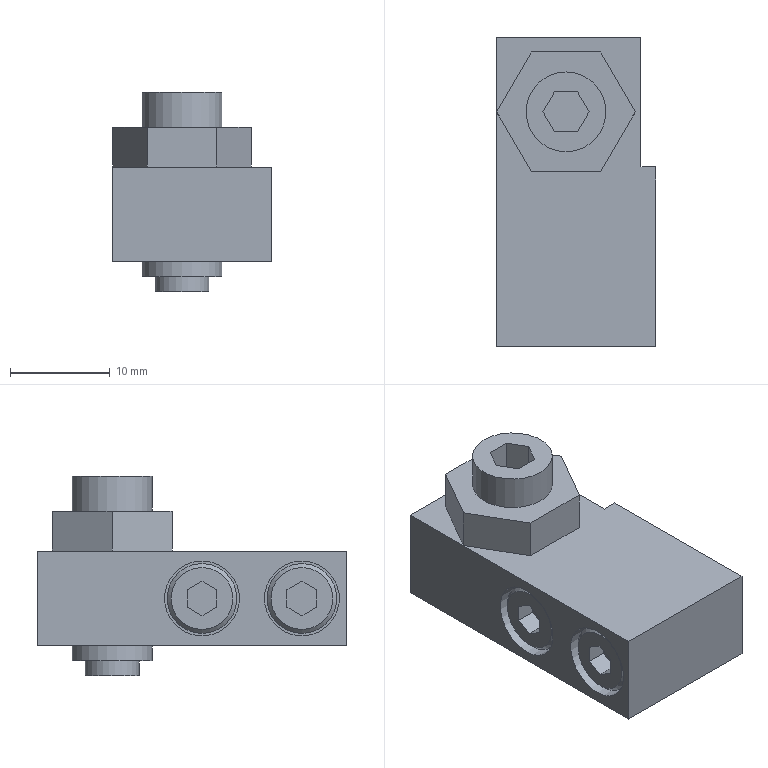Part | NX | 1 solid | 52 faces | box 16 x 31 x 20 mm | volume 5140 mm3 | plane 43 | cylinder 7 | cone 2 | commonest cylinder face diameters 7 x2 7.5 x2 8 x2 5.4 x1
STEP:
#1=CARTESIAN_POINT('',(-40.,0.5,58.5));
#2=VERTEX_POINT('',#1);
#3=CARTESIAN_POINT('',(-24.,0.5,58.5));
#4=VERTEX_POINT('',#3);
#5=CARTESIAN_POINT('',(-24.,0.5,58.5));
#6=DIRECTION('',(1.,0.,0.));
#7=VECTOR('',#6,1000.);
#8=LINE('',#5,#7);
#9=EDGE_CURVE('',#2,#4,#8,.T.);
#10=ORIENTED_EDGE('',*,*,#9,.F.);
#11=CARTESIAN_POINT('',(-40.,31.5,58.5));
#12=VERTEX_POINT('',#11);
#13=CARTESIAN_POINT('',(-40.,0.5,58.5));
#14=DIRECTION('',(0.,1.,0.));
#15=VECTOR('',#14,1000.);
#16=LINE('',#13,#15);
#17=EDGE_CURVE('',#12,#2,#16,.F.);
#18=ORIENTED_EDGE('',*,*,#17,.F.);
#19=CARTESIAN_POINT('',(-25.5,31.5,58.5));
#20=VERTEX_POINT('',#19);
#21=CARTESIAN_POINT('',(-24.,31.5,58.5));
#22=DIRECTION('',(1.,0.,0.));
#23=VECTOR('',#22,1000.);
#24=LINE('',#21,#23);
#25=EDGE_CURVE('',#20,#12,#24,.F.);
#26=ORIENTED_EDGE('',*,*,#25,.F.);
#27=CARTESIAN_POINT('',(-25.5,18.5,58.5));
#28=VERTEX_POINT('',#27);
#29=CARTESIAN_POINT('',(-25.5,0.5,58.5));
#30=DIRECTION('',(0.,1.,0.));
#31=VECTOR('',#30,1000.);
#32=LINE('',#29,#31);
#33=EDGE_CURVE('',#28,#20,#32,.T.);
#34=ORIENTED_EDGE('',*,*,#33,.F.);
#35=CARTESIAN_POINT('',(-24.,18.5,58.5));
#36=VERTEX_POINT('',#35);
#37=CARTESIAN_POINT('',(-24.,18.5,58.5));
#38=DIRECTION('',(1.,0.,0.));
#39=VECTOR('',#38,1000.);
#40=LINE('',#37,#39);
#41=EDGE_CURVE('',#36,#28,#40,.F.);
#42=ORIENTED_EDGE('',*,*,#41,.F.);
#43=CARTESIAN_POINT('',(-24.,0.5,58.5));
#44=DIRECTION('',(0.,1.,0.));
#45=VECTOR('',#44,1000.);
#46=LINE('',#43,#45);
#47=EDGE_CURVE('',#4,#36,#46,.T.);
#48=ORIENTED_EDGE('',*,*,#47,.F.);
#49=EDGE_LOOP('',(#10,#18,#26,#34,#42,#48));
#50=FACE_BOUND('',#49,.T.);
#51=CARTESIAN_POINT('',(-33.,28.,58.5));
#52=VERTEX_POINT('',#51);
#53=CARTESIAN_POINT('',(-33.,24.,58.5));
#54=DIRECTION('',(0.,0.,-1.));
#55=DIRECTION('',(0.,1.,0.));
#56=AXIS2_PLACEMENT_3D('',#53,#54,#55);
#57=CIRCLE('',#56,4.);
#58=EDGE_CURVE('',#52,#52,#57,.T.);
#59=ORIENTED_EDGE('',*,*,#58,.F.);
#60=EDGE_LOOP('',(#59));
#61=FACE_BOUND('',#60,.T.);
#62=CARTESIAN_POINT('',(-24.,0.5,58.5));
#63=DIRECTION('',(0.,0.,1.));
#64=DIRECTION('',(1.,0.,0.));
#65=AXIS2_PLACEMENT_3D('',#62,#63,#64);
#66=PLANE('',#65);
#67=ADVANCED_FACE('',(#50,#61),#66,.F.);
#68=CARTESIAN_POINT('',(-24.,18.5,68.));
#69=VERTEX_POINT('',#68);
#70=CARTESIAN_POINT('',(-24.,0.5,68.));
#71=VERTEX_POINT('',#70);
#72=CARTESIAN_POINT('',(-24.,0.5,68.));
#73=DIRECTION('',(0.,1.,0.));
#74=VECTOR('',#73,1000.);
#75=LINE('',#72,#74);
#76=EDGE_CURVE('',#69,#71,#75,.F.);
#77=ORIENTED_EDGE('',*,*,#76,.T.);
#78=CARTESIAN_POINT('',(-24.,0.5,68.));
#79=DIRECTION('',(0.,0.,-1.));
#80=VECTOR('',#79,1000.);
#81=LINE('',#78,#80);
#82=EDGE_CURVE('',#71,#4,#81,.T.);
#83=ORIENTED_EDGE('',*,*,#82,.T.);
#84=ORIENTED_EDGE('',*,*,#47,.T.);
#85=CARTESIAN_POINT('',(-24.,18.5,68.));
#86=DIRECTION('',(0.,0.,-1.));
#87=VECTOR('',#86,1000.);
#88=LINE('',#85,#87);
#89=EDGE_CURVE('',#36,#69,#88,.F.);
#90=ORIENTED_EDGE('',*,*,#89,.T.);
#91=EDGE_LOOP('',(#77,#83,#84,#90));
#92=FACE_BOUND('',#91,.T.);
#93=CARTESIAN_POINT('',(-24.,0.5,68.));
#94=DIRECTION('',(1.,0.,0.));
#95=DIRECTION('',(0.,0.,-1.));
#96=AXIS2_PLACEMENT_3D('',#93,#94,#95);
#97=PLANE('',#96);
#98=ADVANCED_FACE('',(#92),#97,.T.);
#99=CARTESIAN_POINT('',(-40.,0.5,68.));
#100=VERTEX_POINT('',#99);
#101=CARTESIAN_POINT('',(-40.,0.5,68.));
#102=DIRECTION('',(1.,0.,0.));
#103=VECTOR('',#102,1000.);
#104=LINE('',#101,#103);
#105=EDGE_CURVE('',#71,#100,#104,.F.);
#106=ORIENTED_EDGE('',*,*,#105,.T.);
#107=CARTESIAN_POINT('',(-40.,0.5,68.));
#108=DIRECTION('',(0.,0.,-1.));
#109=VECTOR('',#108,1000.);
#110=LINE('',#107,#109);
#111=EDGE_CURVE('',#100,#2,#110,.T.);
#112=ORIENTED_EDGE('',*,*,#111,.T.);
#113=ORIENTED_EDGE('',*,*,#9,.T.);
#114=ORIENTED_EDGE('',*,*,#82,.F.);
#115=EDGE_LOOP('',(#106,#112,#113,#114));
#116=FACE_BOUND('',#115,.T.);
#117=CARTESIAN_POINT('',(-40.,0.5,68.));
#118=DIRECTION('',(0.,-1.,0.));
#119=DIRECTION('',(0.,0.,-1.));
#120=AXIS2_PLACEMENT_3D('',#117,#118,#119);
#121=PLANE('',#120);
#122=ADVANCED_FACE('',(#116),#121,.T.);
#123=CARTESIAN_POINT('',(-40.,31.5,68.));
#124=VERTEX_POINT('',#123);
#125=CARTESIAN_POINT('',(-40.,31.5,68.));
#126=DIRECTION('',(0.,1.,0.));
#127=VECTOR('',#126,1000.);
#128=LINE('',#125,#127);
#129=EDGE_CURVE('',#100,#124,#128,.T.);
#130=ORIENTED_EDGE('',*,*,#129,.T.);
#131=CARTESIAN_POINT('',(-40.,31.5,68.));
#132=DIRECTION('',(0.,0.,1.));
#133=VECTOR('',#132,1000.);
#134=LINE('',#131,#133);
#135=EDGE_CURVE('',#124,#12,#134,.F.);
#136=ORIENTED_EDGE('',*,*,#135,.T.);
#137=ORIENTED_EDGE('',*,*,#17,.T.);
#138=ORIENTED_EDGE('',*,*,#111,.F.);
#139=EDGE_LOOP('',(#130,#136,#137,#138));
#140=FACE_BOUND('',#139,.T.);
#141=CARTESIAN_POINT('',(-40.,5.,67.));
#142=VERTEX_POINT('',#141);
#143=CARTESIAN_POINT('',(-40.,5.,63.25));
#144=DIRECTION('',(-1.,0.,0.));
#145=DIRECTION('',(0.,0.,1.));
#146=AXIS2_PLACEMENT_3D('',#143,#144,#145);
#147=CIRCLE('',#146,3.75);
#148=EDGE_CURVE('',#142,#142,#147,.F.);
#149=ORIENTED_EDGE('',*,*,#148,.T.);
#150=EDGE_LOOP('',(#149));
#151=FACE_BOUND('',#150,.T.);
#152=CARTESIAN_POINT('',(-40.,15.,67.));
#153=VERTEX_POINT('',#152);
#154=CARTESIAN_POINT('',(-40.,15.,63.25));
#155=DIRECTION('',(-1.,0.,0.));
#156=DIRECTION('',(0.,0.,1.));
#157=AXIS2_PLACEMENT_3D('',#154,#155,#156);
#158=CIRCLE('',#157,3.75);
#159=EDGE_CURVE('',#153,#153,#158,.F.);
#160=ORIENTED_EDGE('',*,*,#159,.T.);
#161=EDGE_LOOP('',(#160));
#162=FACE_BOUND('',#161,.T.);
#163=CARTESIAN_POINT('',(-40.,31.5,68.));
#164=DIRECTION('',(-1.,0.,0.));
#165=DIRECTION('',(0.,0.,1.));
#166=AXIS2_PLACEMENT_3D('',#163,#164,#165);
#167=PLANE('',#166);
#168=ADVANCED_FACE('',(#140,#151,#162),#167,.T.);
#169=CARTESIAN_POINT('',(-25.5,31.5,68.));
#170=VERTEX_POINT('',#169);
#171=CARTESIAN_POINT('',(-25.5,31.5,68.));
#172=DIRECTION('',(1.,0.,0.));
#173=VECTOR('',#172,1000.);
#174=LINE('',#171,#173);
#175=EDGE_CURVE('',#124,#170,#174,.T.);
#176=ORIENTED_EDGE('',*,*,#175,.T.);
#177=CARTESIAN_POINT('',(-25.5,31.5,68.));
#178=DIRECTION('',(0.,0.,1.));
#179=VECTOR('',#178,1000.);
#180=LINE('',#177,#179);
#181=EDGE_CURVE('',#170,#20,#180,.F.);
#182=ORIENTED_EDGE('',*,*,#181,.T.);
#183=ORIENTED_EDGE('',*,*,#25,.T.);
#184=ORIENTED_EDGE('',*,*,#135,.F.);
#185=EDGE_LOOP('',(#176,#182,#183,#184));
#186=FACE_BOUND('',#185,.T.);
#187=CARTESIAN_POINT('',(-25.5,31.5,68.));
#188=DIRECTION('',(0.,1.,0.));
#189=DIRECTION('',(0.,0.,1.));
#190=AXIS2_PLACEMENT_3D('',#187,#188,#189);
#191=PLANE('',#190);
#192=ADVANCED_FACE('',(#186),#191,.T.);
#193=CARTESIAN_POINT('',(-25.5,18.5,68.));
#194=VERTEX_POINT('',#193);
#195=CARTESIAN_POINT('',(-25.5,18.5,68.));
#196=DIRECTION('',(0.,1.,0.));
#197=VECTOR('',#196,1000.);
#198=LINE('',#195,#197);
#199=EDGE_CURVE('',#170,#194,#198,.F.);
#200=ORIENTED_EDGE('',*,*,#199,.T.);
#201=CARTESIAN_POINT('',(-25.5,18.5,68.));
#202=DIRECTION('',(0.,0.,-1.));
#203=VECTOR('',#202,1000.);
#204=LINE('',#201,#203);
#205=EDGE_CURVE('',#194,#28,#204,.T.);
#206=ORIENTED_EDGE('',*,*,#205,.T.);
#207=ORIENTED_EDGE('',*,*,#33,.T.);
#208=ORIENTED_EDGE('',*,*,#181,.F.);
#209=EDGE_LOOP('',(#200,#206,#207,#208));
#210=FACE_BOUND('',#209,.T.);
#211=CARTESIAN_POINT('',(-25.5,18.5,68.));
#212=DIRECTION('',(1.,0.,0.));
#213=DIRECTION('',(0.,0.,-1.));
#214=AXIS2_PLACEMENT_3D('',#211,#212,#213);
#215=PLANE('',#214);
#216=ADVANCED_FACE('',(#210),#215,.T.);
#217=CARTESIAN_POINT('',(-33.,28.,57.));
#218=VERTEX_POINT('',#217);
#219=CARTESIAN_POINT('',(-33.,24.,57.));
#220=DIRECTION('',(0.,0.,-1.));
#221=DIRECTION('',(0.,1.,0.));
#222=AXIS2_PLACEMENT_3D('',#219,#220,#221);
#223=CIRCLE('',#222,4.);
#224=EDGE_CURVE('',#218,#218,#223,.F.);
#225=ORIENTED_EDGE('',*,*,#224,.T.);
#226=EDGE_LOOP('',(#225));
#227=FACE_BOUND('',#226,.T.);
#228=ORIENTED_EDGE('',*,*,#58,.T.);
#229=EDGE_LOOP('',(#228));
#230=FACE_BOUND('',#229,.T.);
#231=CARTESIAN_POINT('',(-33.,24.,66.25));
#232=DIRECTION('',(0.,0.,-1.));
#233=DIRECTION('',(0.,1.,0.));
#234=AXIS2_PLACEMENT_3D('',#231,#232,#233);
#235=CYLINDRICAL_SURFACE('',#234,4.);
#236=ADVANCED_FACE('',(#227,#230),#235,.T.);
#237=ORIENTED_EDGE('',*,*,#175,.F.);
#238=ORIENTED_EDGE('',*,*,#129,.F.);
#239=ORIENTED_EDGE('',*,*,#105,.F.);
#240=ORIENTED_EDGE('',*,*,#76,.F.);
#241=CARTESIAN_POINT('',(-24.,18.5,68.));
#242=DIRECTION('',(1.,0.,0.));
#243=VECTOR('',#242,1000.);
#244=LINE('',#241,#243);
#245=EDGE_CURVE('',#69,#194,#244,.F.);
#246=ORIENTED_EDGE('',*,*,#245,.T.);
#247=ORIENTED_EDGE('',*,*,#199,.F.);
#248=EDGE_LOOP('',(#237,#238,#239,#240,#246,#247));
#249=FACE_BOUND('',#248,.T.);
#250=CARTESIAN_POINT('',(-29.536,18.,68.));
#251=VERTEX_POINT('',#250);
#252=CARTESIAN_POINT('',(-36.464,18.,68.));
#253=VERTEX_POINT('',#252);
#254=CARTESIAN_POINT('',(-24.,18.,68.));
#255=DIRECTION('',(1.,0.,0.));
#256=VECTOR('',#255,1000.);
#257=LINE('',#254,#256);
#258=EDGE_CURVE('',#251,#253,#257,.F.);
#259=ORIENTED_EDGE('',*,*,#258,.T.);
#260=CARTESIAN_POINT('',(-39.928,24.,68.));
#261=VERTEX_POINT('',#260);
#262=CARTESIAN_POINT('',(-36.464,18.,68.));
#263=DIRECTION('',(-0.5,0.866,0.));
#264=VECTOR('',#263,1000.);
#265=LINE('',#262,#264);
#266=EDGE_CURVE('',#253,#261,#265,.T.);
#267=ORIENTED_EDGE('',*,*,#266,.T.);
#268=CARTESIAN_POINT('',(-36.464,30.,68.));
#269=VERTEX_POINT('',#268);
#270=CARTESIAN_POINT('',(-39.928,24.,68.));
#271=DIRECTION('',(0.5,0.866,0.));
#272=VECTOR('',#271,1000.);
#273=LINE('',#270,#272);
#274=EDGE_CURVE('',#261,#269,#273,.T.);
#275=ORIENTED_EDGE('',*,*,#274,.T.);
#276=CARTESIAN_POINT('',(-29.536,30.,68.));
#277=VERTEX_POINT('',#276);
#278=CARTESIAN_POINT('',(-24.,30.,68.));
#279=DIRECTION('',(1.,0.,0.));
#280=VECTOR('',#279,1000.);
#281=LINE('',#278,#280);
#282=EDGE_CURVE('',#269,#277,#281,.T.);
#283=ORIENTED_EDGE('',*,*,#282,.T.);
#284=CARTESIAN_POINT('',(-26.072,24.,68.));
#285=VERTEX_POINT('',#284);
#286=CARTESIAN_POINT('',(-29.536,30.,68.));
#287=DIRECTION('',(0.5,-0.866,0.));
#288=VECTOR('',#287,1000.);
#289=LINE('',#286,#288);
#290=EDGE_CURVE('',#277,#285,#289,.T.);
#291=ORIENTED_EDGE('',*,*,#290,.T.);
#292=CARTESIAN_POINT('',(-26.072,24.,68.));
#293=DIRECTION('',(-0.5,-0.866,0.));
#294=VECTOR('',#293,1000.);
#295=LINE('',#292,#294);
#296=EDGE_CURVE('',#285,#251,#295,.T.);
#297=ORIENTED_EDGE('',*,*,#296,.T.);
#298=EDGE_LOOP('',(#259,#267,#275,#283,#291,#297));
#299=FACE_BOUND('',#298,.T.);
#300=CARTESIAN_POINT('',(-24.,0.5,68.));
#301=DIRECTION('',(0.,0.,1.));
#302=DIRECTION('',(1.,0.,0.));
#303=AXIS2_PLACEMENT_3D('',#300,#301,#302);
#304=PLANE('',#303);
#305=ADVANCED_FACE('',(#249,#299),#304,.T.);
#306=ORIENTED_EDGE('',*,*,#245,.F.);
#307=ORIENTED_EDGE('',*,*,#89,.F.);
#308=ORIENTED_EDGE('',*,*,#41,.T.);
#309=ORIENTED_EDGE('',*,*,#205,.F.);
#310=EDGE_LOOP('',(#306,#307,#308,#309));
#311=FACE_BOUND('',#310,.T.);
#312=CARTESIAN_POINT('',(-24.,18.5,68.));
#313=DIRECTION('',(0.,1.,0.));
#314=DIRECTION('',(0.,0.,1.));
#315=AXIS2_PLACEMENT_3D('',#312,#313,#314);
#316=PLANE('',#315);
#317=ADVANCED_FACE('',(#311),#316,.T.);
#318=ORIENTED_EDGE('',*,*,#148,.F.);
#319=EDGE_LOOP('',(#318));
#320=FACE_BOUND('',#319,.T.);
#321=CARTESIAN_POINT('',(-35.6,5.,67.));
#322=VERTEX_POINT('',#321);
#323=CARTESIAN_POINT('',(-35.6,5.,63.25));
#324=DIRECTION('',(-1.,0.,0.));
#325=DIRECTION('',(0.,0.,1.));
#326=AXIS2_PLACEMENT_3D('',#323,#324,#325);
#327=CIRCLE('',#326,3.75);
#328=EDGE_CURVE('',#322,#322,#327,.T.);
#329=ORIENTED_EDGE('',*,*,#328,.F.);
#330=EDGE_LOOP('',(#329));
#331=FACE_BOUND('',#330,.T.);
#332=CARTESIAN_POINT('',(-40.,5.,63.25));
#333=DIRECTION('',(-1.,0.,0.));
#334=DIRECTION('',(0.,0.,1.));
#335=AXIS2_PLACEMENT_3D('',#332,#333,#334);
#336=CYLINDRICAL_SURFACE('',#335,3.75);
#337=ADVANCED_FACE('',(#320,#331),#336,.F.);
#338=ORIENTED_EDGE('',*,*,#159,.F.);
#339=EDGE_LOOP('',(#338));
#340=FACE_BOUND('',#339,.T.);
#341=CARTESIAN_POINT('',(-35.6,15.,67.));
#342=VERTEX_POINT('',#341);
#343=CARTESIAN_POINT('',(-35.6,15.,63.25));
#344=DIRECTION('',(-1.,0.,0.));
#345=DIRECTION('',(0.,0.,1.));
#346=AXIS2_PLACEMENT_3D('',#343,#344,#345);
#347=CIRCLE('',#346,3.75);
#348=EDGE_CURVE('',#342,#342,#347,.T.);
#349=ORIENTED_EDGE('',*,*,#348,.F.);
#350=EDGE_LOOP('',(#349));
#351=FACE_BOUND('',#350,.T.);
#352=CARTESIAN_POINT('',(-40.,15.,63.25));
#353=DIRECTION('',(-1.,0.,0.));
#354=DIRECTION('',(0.,0.,1.));
#355=AXIS2_PLACEMENT_3D('',#352,#353,#354);
#356=CYLINDRICAL_SURFACE('',#355,3.75);
#357=ADVANCED_FACE('',(#340,#351),#356,.F.);
#358=CARTESIAN_POINT('',(-33.,26.7,57.));
#359=VERTEX_POINT('',#358);
#360=CARTESIAN_POINT('',(-33.,24.,57.));
#361=DIRECTION('',(0.,0.,-1.));
#362=DIRECTION('',(0.,1.,0.));
#363=AXIS2_PLACEMENT_3D('',#360,#361,#362);
#364=CIRCLE('',#363,2.7);
#365=EDGE_CURVE('',#359,#359,#364,.F.);
#366=ORIENTED_EDGE('',*,*,#365,.T.);
#367=EDGE_LOOP('',(#366));
#368=FACE_BOUND('',#367,.T.);
#369=ORIENTED_EDGE('',*,*,#224,.F.);
#370=EDGE_LOOP('',(#369));
#371=FACE_BOUND('',#370,.T.);
#372=CARTESIAN_POINT('',(-33.,27.35,57.));
#373=DIRECTION('',(0.,0.,-1.));
#374=DIRECTION('',(-1.,0.,0.));
#375=AXIS2_PLACEMENT_3D('',#372,#373,#374);
#376=PLANE('',#375);
#377=ADVANCED_FACE('',(#368,#371),#376,.T.);
#378=ORIENTED_EDGE('',*,*,#266,.F.);
#379=CARTESIAN_POINT('',(-36.464,18.,72.));
#380=VERTEX_POINT('',#379);
#381=CARTESIAN_POINT('',(-36.464,18.,68.));
#382=DIRECTION('',(0.,0.,1.));
#383=VECTOR('',#382,1000.);
#384=LINE('',#381,#383);
#385=EDGE_CURVE('',#253,#380,#384,.T.);
#386=ORIENTED_EDGE('',*,*,#385,.T.);
#387=CARTESIAN_POINT('',(-39.928,24.,72.));
#388=VERTEX_POINT('',#387);
#389=CARTESIAN_POINT('',(-36.464,18.,72.));
#390=DIRECTION('',(0.5,-0.866,0.));
#391=VECTOR('',#390,1000.);
#392=LINE('',#389,#391);
#393=EDGE_CURVE('',#380,#388,#392,.F.);
#394=ORIENTED_EDGE('',*,*,#393,.T.);
#395=CARTESIAN_POINT('',(-39.928,24.,68.));
#396=DIRECTION('',(0.,0.,1.));
#397=VECTOR('',#396,1000.);
#398=LINE('',#395,#397);
#399=EDGE_CURVE('',#388,#261,#398,.F.);
#400=ORIENTED_EDGE('',*,*,#399,.T.);
#401=EDGE_LOOP('',(#378,#386,#394,#400));
#402=FACE_BOUND('',#401,.T.);
#403=CARTESIAN_POINT('',(-36.464,18.,68.));
#404=DIRECTION('',(-0.866,-0.5,0.));
#405=DIRECTION('',(0.5,-0.866,0.));
#406=AXIS2_PLACEMENT_3D('',#403,#404,#405);
#407=PLANE('',#406);
#408=ADVANCED_FACE('',(#402),#407,.T.);
#409=ORIENTED_EDGE('',*,*,#258,.F.);
#410=CARTESIAN_POINT('',(-29.536,18.,72.));
#411=VERTEX_POINT('',#410);
#412=CARTESIAN_POINT('',(-29.536,18.,68.));
#413=DIRECTION('',(0.,0.,1.));
#414=VECTOR('',#413,1000.);
#415=LINE('',#412,#414);
#416=EDGE_CURVE('',#251,#411,#415,.T.);
#417=ORIENTED_EDGE('',*,*,#416,.T.);
#418=CARTESIAN_POINT('',(-29.536,18.,72.));
#419=DIRECTION('',(1.,0.,0.));
#420=VECTOR('',#419,1000.);
#421=LINE('',#418,#420);
#422=EDGE_CURVE('',#411,#380,#421,.F.);
#423=ORIENTED_EDGE('',*,*,#422,.T.);
#424=ORIENTED_EDGE('',*,*,#385,.F.);
#425=EDGE_LOOP('',(#409,#417,#423,#424));
#426=FACE_BOUND('',#425,.T.);
#427=CARTESIAN_POINT('',(-29.536,18.,68.));
#428=DIRECTION('',(0.,-1.,0.));
#429=DIRECTION('',(1.,0.,0.));
#430=AXIS2_PLACEMENT_3D('',#427,#428,#429);
#431=PLANE('',#430);
#432=ADVANCED_FACE('',(#426),#431,.T.);
#433=ORIENTED_EDGE('',*,*,#296,.F.);
#434=CARTESIAN_POINT('',(-26.072,24.,72.));
#435=VERTEX_POINT('',#434);
#436=CARTESIAN_POINT('',(-26.072,24.,68.));
#437=DIRECTION('',(0.,0.,1.));
#438=VECTOR('',#437,1000.);
#439=LINE('',#436,#438);
#440=EDGE_CURVE('',#285,#435,#439,.T.);
#441=ORIENTED_EDGE('',*,*,#440,.T.);
#442=CARTESIAN_POINT('',(-26.072,24.,72.));
#443=DIRECTION('',(0.5,0.866,0.));
#444=VECTOR('',#443,1000.);
#445=LINE('',#442,#444);
#446=EDGE_CURVE('',#435,#411,#445,.F.);
#447=ORIENTED_EDGE('',*,*,#446,.T.);
#448=ORIENTED_EDGE('',*,*,#416,.F.);
#449=EDGE_LOOP('',(#433,#441,#447,#448));
#450=FACE_BOUND('',#449,.T.);
#451=CARTESIAN_POINT('',(-26.072,24.,68.));
#452=DIRECTION('',(0.866,-0.5,0.));
#453=DIRECTION('',(0.5,0.866,0.));
#454=AXIS2_PLACEMENT_3D('',#451,#452,#453);
#455=PLANE('',#454);
#456=ADVANCED_FACE('',(#450),#455,.T.);
#457=ORIENTED_EDGE('',*,*,#290,.F.);
#458=CARTESIAN_POINT('',(-29.536,30.,72.));
#459=VERTEX_POINT('',#458);
#460=CARTESIAN_POINT('',(-29.536,30.,68.));
#461=DIRECTION('',(0.,0.,1.));
#462=VECTOR('',#461,1000.);
#463=LINE('',#460,#462);
#464=EDGE_CURVE('',#277,#459,#463,.T.);
#465=ORIENTED_EDGE('',*,*,#464,.T.);
#466=CARTESIAN_POINT('',(-29.536,30.,72.));
#467=DIRECTION('',(-0.5,0.866,0.));
#468=VECTOR('',#467,1000.);
#469=LINE('',#466,#468);
#470=EDGE_CURVE('',#459,#435,#469,.F.);
#471=ORIENTED_EDGE('',*,*,#470,.T.);
#472=ORIENTED_EDGE('',*,*,#440,.F.);
#473=EDGE_LOOP('',(#457,#465,#471,#472));
#474=FACE_BOUND('',#473,.T.);
#475=CARTESIAN_POINT('',(-29.536,30.,68.));
#476=DIRECTION('',(0.866,0.5,0.));
#477=DIRECTION('',(-0.5,0.866,0.));
#478=AXIS2_PLACEMENT_3D('',#475,#476,#477);
#479=PLANE('',#478);
#480=ADVANCED_FACE('',(#474),#479,.T.);
#481=ORIENTED_EDGE('',*,*,#282,.F.);
#482=CARTESIAN_POINT('',(-36.464,30.,72.));
#483=VERTEX_POINT('',#482);
#484=CARTESIAN_POINT('',(-36.464,30.,68.));
#485=DIRECTION('',(0.,0.,1.));
#486=VECTOR('',#485,1000.);
#487=LINE('',#484,#486);
#488=EDGE_CURVE('',#269,#483,#487,.T.);
#489=ORIENTED_EDGE('',*,*,#488,.T.);
#490=CARTESIAN_POINT('',(-36.464,30.,72.));
#491=DIRECTION('',(-1.,0.,0.));
#492=VECTOR('',#491,1000.);
#493=LINE('',#490,#492);
#494=EDGE_CURVE('',#483,#459,#493,.F.);
#495=ORIENTED_EDGE('',*,*,#494,.T.);
#496=ORIENTED_EDGE('',*,*,#464,.F.);
#497=EDGE_LOOP('',(#481,#489,#495,#496));
#498=FACE_BOUND('',#497,.T.);
#499=CARTESIAN_POINT('',(-36.464,30.,68.));
#500=DIRECTION('',(0.,1.,0.));
#501=DIRECTION('',(-1.,0.,0.));
#502=AXIS2_PLACEMENT_3D('',#499,#500,#501);
#503=PLANE('',#502);
#504=ADVANCED_FACE('',(#498),#503,.T.);
#505=ORIENTED_EDGE('',*,*,#274,.F.);
#506=ORIENTED_EDGE('',*,*,#399,.F.);
#507=CARTESIAN_POINT('',(-39.928,24.,72.));
#508=DIRECTION('',(-0.5,-0.866,0.));
#509=VECTOR('',#508,1000.);
#510=LINE('',#507,#509);
#511=EDGE_CURVE('',#388,#483,#510,.F.);
#512=ORIENTED_EDGE('',*,*,#511,.T.);
#513=ORIENTED_EDGE('',*,*,#488,.F.);
#514=EDGE_LOOP('',(#505,#506,#512,#513));
#515=FACE_BOUND('',#514,.T.);
#516=CARTESIAN_POINT('',(-39.928,24.,68.));
#517=DIRECTION('',(-0.866,0.5,0.));
#518=DIRECTION('',(-0.5,-0.866,0.));
#519=AXIS2_PLACEMENT_3D('',#516,#517,#518);
#520=PLANE('',#519);
#521=ADVANCED_FACE('',(#515),#520,.T.);
#522=ORIENTED_EDGE('',*,*,#328,.T.);
#523=EDGE_LOOP('',(#522));
#524=FACE_BOUND('',#523,.T.);
#525=CARTESIAN_POINT('',(-35.6,5.,66.75));
#526=VERTEX_POINT('',#525);
#527=CARTESIAN_POINT('',(-35.6,5.,63.25));
#528=DIRECTION('',(-1.,0.,0.));
#529=DIRECTION('',(0.,0.,1.));
#530=AXIS2_PLACEMENT_3D('',#527,#528,#529);
#531=CIRCLE('',#530,3.5);
#532=EDGE_CURVE('',#526,#526,#531,.T.);
#533=ORIENTED_EDGE('',*,*,#532,.F.);
#534=EDGE_LOOP('',(#533));
#535=FACE_BOUND('',#534,.T.);
#536=CARTESIAN_POINT('',(-35.6,0.5,63.25));
#537=DIRECTION('',(1.,0.,0.));
#538=DIRECTION('',(0.,0.,-1.));
#539=AXIS2_PLACEMENT_3D('',#536,#537,#538);
#540=PLANE('',#539);
#541=ADVANCED_FACE('',(#524,#535),#540,.F.);
#542=ORIENTED_EDGE('',*,*,#348,.T.);
#543=EDGE_LOOP('',(#542));
#544=FACE_BOUND('',#543,.T.);
#545=CARTESIAN_POINT('',(-35.6,15.,66.75));
#546=VERTEX_POINT('',#545);
#547=CARTESIAN_POINT('',(-35.6,15.,63.25));
#548=DIRECTION('',(-1.,0.,0.));
#549=DIRECTION('',(0.,0.,1.));
#550=AXIS2_PLACEMENT_3D('',#547,#548,#549);
#551=CIRCLE('',#550,3.5);
#552=EDGE_CURVE('',#546,#546,#551,.T.);
#553=ORIENTED_EDGE('',*,*,#552,.F.);
#554=EDGE_LOOP('',(#553));
#555=FACE_BOUND('',#554,.T.);
#556=CARTESIAN_POINT('',(-35.6,10.5,63.25));
#557=DIRECTION('',(1.,0.,0.));
#558=DIRECTION('',(0.,0.,-1.));
#559=AXIS2_PLACEMENT_3D('',#556,#557,#558);
#560=PLANE('',#559);
#561=ADVANCED_FACE('',(#544,#555),#560,.F.);
#562=ORIENTED_EDGE('',*,*,#365,.F.);
#563=EDGE_LOOP('',(#562));
#564=FACE_BOUND('',#563,.T.);
#565=CARTESIAN_POINT('',(-33.,26.7,55.5));
#566=VERTEX_POINT('',#565);
#567=CARTESIAN_POINT('',(-33.,24.,55.5));
#568=DIRECTION('',(0.,0.,-1.));
#569=DIRECTION('',(0.,1.,0.));
#570=AXIS2_PLACEMENT_3D('',#567,#568,#569);
#571=CIRCLE('',#570,2.7);
#572=EDGE_CURVE('',#566,#566,#571,.F.);
#573=ORIENTED_EDGE('',*,*,#572,.T.);
#574=EDGE_LOOP('',(#573));
#575=FACE_BOUND('',#574,.T.);
#576=CARTESIAN_POINT('',(-33.,24.,56.25));
#577=DIRECTION('',(0.,0.,-1.));
#578=DIRECTION('',(0.,1.,0.));
#579=AXIS2_PLACEMENT_3D('',#576,#577,#578);
#580=CYLINDRICAL_SURFACE('',#579,2.7);
#581=ADVANCED_FACE('',(#564,#575),#580,.T.);
#582=CARTESIAN_POINT('',(-33.,28.,72.));
#583=VERTEX_POINT('',#582);
#584=CARTESIAN_POINT('',(-33.,24.,72.));
#585=DIRECTION('',(0.,0.,-1.));
#586=DIRECTION('',(0.,1.,0.));
#587=AXIS2_PLACEMENT_3D('',#584,#585,#586);
#588=CIRCLE('',#587,4.);
#589=EDGE_CURVE('',#583,#583,#588,.T.);
#590=ORIENTED_EDGE('',*,*,#589,.T.);
#591=EDGE_LOOP('',(#590));
#592=FACE_BOUND('',#591,.T.);
#593=ORIENTED_EDGE('',*,*,#470,.F.);
#594=ORIENTED_EDGE('',*,*,#494,.F.);
#595=ORIENTED_EDGE('',*,*,#511,.F.);
#596=ORIENTED_EDGE('',*,*,#393,.F.);
#597=ORIENTED_EDGE('',*,*,#422,.F.);
#598=ORIENTED_EDGE('',*,*,#446,.F.);
#599=EDGE_LOOP('',(#593,#594,#595,#596,#597,#598));
#600=FACE_BOUND('',#599,.T.);
#601=CARTESIAN_POINT('',(-24.,0.5,72.));
#602=DIRECTION('',(0.,0.,1.));
#603=DIRECTION('',(1.,0.,0.));
#604=AXIS2_PLACEMENT_3D('',#601,#602,#603);
#605=PLANE('',#604);
#606=ADVANCED_FACE('',(#592,#600),#605,.T.);
#607=CARTESIAN_POINT('',(-39.2,5.,66.75));
#608=VERTEX_POINT('',#607);
#609=CARTESIAN_POINT('',(-39.2,5.,63.25));
#610=DIRECTION('',(-1.,0.,0.));
#611=DIRECTION('',(0.,0.,1.));
#612=AXIS2_PLACEMENT_3D('',#609,#610,#611);
#613=CIRCLE('',#612,3.5);
#614=EDGE_CURVE('',#608,#608,#613,.F.);
#615=ORIENTED_EDGE('',*,*,#614,.T.);
#616=EDGE_LOOP('',(#615));
#617=FACE_BOUND('',#616,.T.);
#618=ORIENTED_EDGE('',*,*,#532,.T.);
#619=EDGE_LOOP('',(#618));
#620=FACE_BOUND('',#619,.T.);
#621=CARTESIAN_POINT('',(-37.4,5.,63.25));
#622=DIRECTION('',(-1.,0.,0.));
#623=DIRECTION('',(0.,0.,1.));
#624=AXIS2_PLACEMENT_3D('',#621,#622,#623);
#625=CYLINDRICAL_SURFACE('',#624,3.5);
#626=ADVANCED_FACE('',(#617,#620),#625,.T.);
#627=CARTESIAN_POINT('',(-39.2,15.,66.75));
#628=VERTEX_POINT('',#627);
#629=CARTESIAN_POINT('',(-39.2,15.,63.25));
#630=DIRECTION('',(-1.,0.,0.));
#631=DIRECTION('',(0.,0.,1.));
#632=AXIS2_PLACEMENT_3D('',#629,#630,#631);
#633=CIRCLE('',#632,3.5);
#634=EDGE_CURVE('',#628,#628,#633,.F.);
#635=ORIENTED_EDGE('',*,*,#634,.T.);
#636=EDGE_LOOP('',(#635));
#637=FACE_BOUND('',#636,.T.);
#638=ORIENTED_EDGE('',*,*,#552,.T.);
#639=EDGE_LOOP('',(#638));
#640=FACE_BOUND('',#639,.T.);
#641=CARTESIAN_POINT('',(-37.4,15.,63.25));
#642=DIRECTION('',(-1.,0.,0.));
#643=DIRECTION('',(0.,0.,1.));
#644=AXIS2_PLACEMENT_3D('',#641,#642,#643);
#645=CYLINDRICAL_SURFACE('',#644,3.5);
#646=ADVANCED_FACE('',(#637,#640),#645,.T.);
#647=ORIENTED_EDGE('',*,*,#572,.F.);
#648=EDGE_LOOP('',(#647));
#649=FACE_BOUND('',#648,.T.);
#650=CARTESIAN_POINT('',(-33.,25.35,55.5));
#651=DIRECTION('',(0.,0.,-1.));
#652=DIRECTION('',(-1.,0.,0.));
#653=AXIS2_PLACEMENT_3D('',#650,#651,#652);
#654=PLANE('',#653);
#655=ADVANCED_FACE('',(#649),#654,.T.);
#656=ORIENTED_EDGE('',*,*,#589,.F.);
#657=EDGE_LOOP('',(#656));
#658=FACE_BOUND('',#657,.T.);
#659=CARTESIAN_POINT('',(-33.,28.,75.5));
#660=VERTEX_POINT('',#659);
#661=CARTESIAN_POINT('',(-33.,24.,75.5));
#662=DIRECTION('',(0.,0.,-1.));
#663=DIRECTION('',(0.,1.,0.));
#664=AXIS2_PLACEMENT_3D('',#661,#662,#663);
#665=CIRCLE('',#664,4.);
#666=EDGE_CURVE('',#660,#660,#665,.T.);
#667=ORIENTED_EDGE('',*,*,#666,.T.);
#668=EDGE_LOOP('',(#667));
#669=FACE_BOUND('',#668,.T.);
#670=CARTESIAN_POINT('',(-33.,24.,66.25));
#671=DIRECTION('',(0.,0.,-1.));
#672=DIRECTION('',(0.,1.,0.));
#673=AXIS2_PLACEMENT_3D('',#670,#671,#672);
#674=CYLINDRICAL_SURFACE('',#673,4.);
#675=ADVANCED_FACE('',(#658,#669),#674,.T.);
#676=CARTESIAN_POINT('',(-39.6,5.,60.15));
#677=VERTEX_POINT('',#676);
#678=CARTESIAN_POINT('',(-39.6,5.,63.25));
#679=DIRECTION('',(1.,0.,0.));
#680=DIRECTION('',(0.,0.,-1.));
#681=AXIS2_PLACEMENT_3D('',#678,#679,#680);
#682=CIRCLE('',#681,3.1);
#683=EDGE_CURVE('',#677,#677,#682,.T.);
#684=ORIENTED_EDGE('',*,*,#683,.T.);
#685=EDGE_LOOP('',(#684));
#686=FACE_BOUND('',#685,.T.);
#687=ORIENTED_EDGE('',*,*,#614,.F.);
#688=EDGE_LOOP('',(#687));
#689=FACE_BOUND('',#688,.T.);
#690=CARTESIAN_POINT('',(-39.2,5.,63.25));
#691=DIRECTION('',(1.,0.,0.));
#692=DIRECTION('',(0.,0.,-1.));
#693=AXIS2_PLACEMENT_3D('',#690,#691,#692);
#694=CONICAL_SURFACE('',#693,3.5,0.7854);
#695=ADVANCED_FACE('',(#686,#689),#694,.T.);
#696=CARTESIAN_POINT('',(-39.6,15.,60.15));
#697=VERTEX_POINT('',#696);
#698=CARTESIAN_POINT('',(-39.6,15.,63.25));
#699=DIRECTION('',(1.,0.,0.));
#700=DIRECTION('',(0.,0.,-1.));
#701=AXIS2_PLACEMENT_3D('',#698,#699,#700);
#702=CIRCLE('',#701,3.1);
#703=EDGE_CURVE('',#697,#697,#702,.T.);
#704=ORIENTED_EDGE('',*,*,#703,.T.);
#705=EDGE_LOOP('',(#704));
#706=FACE_BOUND('',#705,.T.);
#707=ORIENTED_EDGE('',*,*,#634,.F.);
#708=EDGE_LOOP('',(#707));
#709=FACE_BOUND('',#708,.T.);
#710=CARTESIAN_POINT('',(-39.2,15.,63.25));
#711=DIRECTION('',(1.,0.,0.));
#712=DIRECTION('',(0.,0.,-1.));
#713=AXIS2_PLACEMENT_3D('',#710,#711,#712);
#714=CONICAL_SURFACE('',#713,3.5,0.7854);
#715=ADVANCED_FACE('',(#706,#709),#714,.T.);
#716=ORIENTED_EDGE('',*,*,#666,.F.);
#717=EDGE_LOOP('',(#716));
#718=FACE_BOUND('',#717,.T.);
#719=CARTESIAN_POINT('',(-31.846,26.,75.5));
#720=VERTEX_POINT('',#719);
#721=CARTESIAN_POINT('',(-30.691,24.,75.5));
#722=VERTEX_POINT('',#721);
#723=CARTESIAN_POINT('',(-31.846,26.,75.5));
#724=DIRECTION('',(0.5,-0.866,0.));
#725=VECTOR('',#724,1000.);
#726=LINE('',#723,#725);
#727=EDGE_CURVE('',#720,#722,#726,.T.);
#728=ORIENTED_EDGE('',*,*,#727,.T.);
#729=CARTESIAN_POINT('',(-31.846,22.,75.5));
#730=VERTEX_POINT('',#729);
#731=CARTESIAN_POINT('',(-30.691,24.,75.5));
#732=DIRECTION('',(-0.5,-0.866,0.));
#733=VECTOR('',#732,1000.);
#734=LINE('',#731,#733);
#735=EDGE_CURVE('',#722,#730,#734,.T.);
#736=ORIENTED_EDGE('',*,*,#735,.T.);
#737=CARTESIAN_POINT('',(-34.154,22.,75.5));
#738=VERTEX_POINT('',#737);
#739=CARTESIAN_POINT('',(-33.,22.,75.5));
#740=DIRECTION('',(1.,0.,0.));
#741=VECTOR('',#740,1000.);
#742=LINE('',#739,#741);
#743=EDGE_CURVE('',#730,#738,#742,.F.);
#744=ORIENTED_EDGE('',*,*,#743,.T.);
#745=CARTESIAN_POINT('',(-35.309,24.,75.5));
#746=VERTEX_POINT('',#745);
#747=CARTESIAN_POINT('',(-34.154,22.,75.5));
#748=DIRECTION('',(-0.5,0.866,0.));
#749=VECTOR('',#748,1000.);
#750=LINE('',#747,#749);
#751=EDGE_CURVE('',#738,#746,#750,.T.);
#752=ORIENTED_EDGE('',*,*,#751,.T.);
#753=CARTESIAN_POINT('',(-34.154,26.,75.5));
#754=VERTEX_POINT('',#753);
#755=CARTESIAN_POINT('',(-35.309,24.,75.5));
#756=DIRECTION('',(0.5,0.866,0.));
#757=VECTOR('',#756,1000.);
#758=LINE('',#755,#757);
#759=EDGE_CURVE('',#746,#754,#758,.T.);
#760=ORIENTED_EDGE('',*,*,#759,.T.);
#761=CARTESIAN_POINT('',(-33.,26.,75.5));
#762=DIRECTION('',(1.,0.,0.));
#763=VECTOR('',#762,1000.);
#764=LINE('',#761,#763);
#765=EDGE_CURVE('',#754,#720,#764,.T.);
#766=ORIENTED_EDGE('',*,*,#765,.T.);
#767=EDGE_LOOP('',(#728,#736,#744,#752,#760,#766));
#768=FACE_BOUND('',#767,.T.);
#769=CARTESIAN_POINT('',(-33.,26.,75.5));
#770=DIRECTION('',(0.,0.,1.));
#771=DIRECTION('',(1.,0.,0.));
#772=AXIS2_PLACEMENT_3D('',#769,#770,#771);
#773=PLANE('',#772);
#774=ADVANCED_FACE('',(#718,#768),#773,.T.);
#775=ORIENTED_EDGE('',*,*,#683,.F.);
#776=EDGE_LOOP('',(#775));
#777=FACE_BOUND('',#776,.T.);
#778=CARTESIAN_POINT('',(-39.6,5.,61.518));
#779=VERTEX_POINT('',#778);
#780=CARTESIAN_POINT('',(-39.6,6.5,62.384));
#781=VERTEX_POINT('',#780);
#782=CARTESIAN_POINT('',(-39.6,6.5,62.384));
#783=DIRECTION('',(0.,0.866,0.5));
#784=VECTOR('',#783,1000.);
#785=LINE('',#782,#784);
#786=EDGE_CURVE('',#779,#781,#785,.T.);
#787=ORIENTED_EDGE('',*,*,#786,.T.);
#788=CARTESIAN_POINT('',(-39.6,6.5,64.116));
#789=VERTEX_POINT('',#788);
#790=CARTESIAN_POINT('',(-39.6,6.5,63.25));
#791=DIRECTION('',(0.,0.,1.));
#792=VECTOR('',#791,1000.);
#793=LINE('',#790,#792);
#794=EDGE_CURVE('',#781,#789,#793,.T.);
#795=ORIENTED_EDGE('',*,*,#794,.T.);
#796=CARTESIAN_POINT('',(-39.6,5.,64.982));
#797=VERTEX_POINT('',#796);
#798=CARTESIAN_POINT('',(-39.6,5.,64.982));
#799=DIRECTION('',(0.,-0.866,0.5));
#800=VECTOR('',#799,1000.);
#801=LINE('',#798,#800);
#802=EDGE_CURVE('',#789,#797,#801,.T.);
#803=ORIENTED_EDGE('',*,*,#802,.T.);
#804=CARTESIAN_POINT('',(-39.6,3.5,64.116));
#805=VERTEX_POINT('',#804);
#806=CARTESIAN_POINT('',(-39.6,3.5,64.116));
#807=DIRECTION('',(0.,-0.866,-0.5));
#808=VECTOR('',#807,1000.);
#809=LINE('',#806,#808);
#810=EDGE_CURVE('',#797,#805,#809,.T.);
#811=ORIENTED_EDGE('',*,*,#810,.T.);
#812=CARTESIAN_POINT('',(-39.6,3.5,62.384));
#813=VERTEX_POINT('',#812);
#814=CARTESIAN_POINT('',(-39.6,3.5,62.384));
#815=DIRECTION('',(0.,0.,-1.));
#816=VECTOR('',#815,1000.);
#817=LINE('',#814,#816);
#818=EDGE_CURVE('',#805,#813,#817,.T.);
#819=ORIENTED_EDGE('',*,*,#818,.T.);
#820=CARTESIAN_POINT('',(-39.6,5.,61.518));
#821=DIRECTION('',(0.,0.866,-0.5));
#822=VECTOR('',#821,1000.);
#823=LINE('',#820,#822);
#824=EDGE_CURVE('',#813,#779,#823,.T.);
#825=ORIENTED_EDGE('',*,*,#824,.T.);
#826=EDGE_LOOP('',(#787,#795,#803,#811,#819,#825));
#827=FACE_BOUND('',#826,.T.);
#828=CARTESIAN_POINT('',(-39.6,3.45,63.25));
#829=DIRECTION('',(-1.,0.,0.));
#830=DIRECTION('',(0.,-1.,0.));
#831=AXIS2_PLACEMENT_3D('',#828,#829,#830);
#832=PLANE('',#831);
#833=ADVANCED_FACE('',(#777,#827),#832,.T.);
#834=ORIENTED_EDGE('',*,*,#703,.F.);
#835=EDGE_LOOP('',(#834));
#836=FACE_BOUND('',#835,.T.);
#837=CARTESIAN_POINT('',(-39.6,15.,61.518));
#838=VERTEX_POINT('',#837);
#839=CARTESIAN_POINT('',(-39.6,16.5,62.384));
#840=VERTEX_POINT('',#839);
#841=CARTESIAN_POINT('',(-39.6,16.5,62.384));
#842=DIRECTION('',(0.,0.866,0.5));
#843=VECTOR('',#842,1000.);
#844=LINE('',#841,#843);
#845=EDGE_CURVE('',#838,#840,#844,.T.);
#846=ORIENTED_EDGE('',*,*,#845,.T.);
#847=CARTESIAN_POINT('',(-39.6,16.5,64.116));
#848=VERTEX_POINT('',#847);
#849=CARTESIAN_POINT('',(-39.6,16.5,63.25));
#850=DIRECTION('',(0.,0.,1.));
#851=VECTOR('',#850,1000.);
#852=LINE('',#849,#851);
#853=EDGE_CURVE('',#840,#848,#852,.T.);
#854=ORIENTED_EDGE('',*,*,#853,.T.);
#855=CARTESIAN_POINT('',(-39.6,15.,64.982));
#856=VERTEX_POINT('',#855);
#857=CARTESIAN_POINT('',(-39.6,15.,64.982));
#858=DIRECTION('',(0.,-0.866,0.5));
#859=VECTOR('',#858,1000.);
#860=LINE('',#857,#859);
#861=EDGE_CURVE('',#848,#856,#860,.T.);
#862=ORIENTED_EDGE('',*,*,#861,.T.);
#863=CARTESIAN_POINT('',(-39.6,13.5,64.116));
#864=VERTEX_POINT('',#863);
#865=CARTESIAN_POINT('',(-39.6,13.5,64.116));
#866=DIRECTION('',(0.,-0.866,-0.5));
#867=VECTOR('',#866,1000.);
#868=LINE('',#865,#867);
#869=EDGE_CURVE('',#856,#864,#868,.T.);
#870=ORIENTED_EDGE('',*,*,#869,.T.);
#871=CARTESIAN_POINT('',(-39.6,13.5,62.384));
#872=VERTEX_POINT('',#871);
#873=CARTESIAN_POINT('',(-39.6,13.5,62.384));
#874=DIRECTION('',(0.,0.,-1.));
#875=VECTOR('',#874,1000.);
#876=LINE('',#873,#875);
#877=EDGE_CURVE('',#864,#872,#876,.T.);
#878=ORIENTED_EDGE('',*,*,#877,.T.);
#879=CARTESIAN_POINT('',(-39.6,15.,61.518));
#880=DIRECTION('',(0.,0.866,-0.5));
#881=VECTOR('',#880,1000.);
#882=LINE('',#879,#881);
#883=EDGE_CURVE('',#872,#838,#882,.T.);
#884=ORIENTED_EDGE('',*,*,#883,.T.);
#885=EDGE_LOOP('',(#846,#854,#862,#870,#878,#884));
#886=FACE_BOUND('',#885,.T.);
#887=CARTESIAN_POINT('',(-39.6,13.45,63.25));
#888=DIRECTION('',(-1.,0.,0.));
#889=DIRECTION('',(0.,-1.,0.));
#890=AXIS2_PLACEMENT_3D('',#887,#888,#889);
#891=PLANE('',#890);
#892=ADVANCED_FACE('',(#836,#886),#891,.T.);
#893=CARTESIAN_POINT('',(-31.846,22.,71.5));
#894=VERTEX_POINT('',#893);
#895=CARTESIAN_POINT('',(-31.846,22.,75.5));
#896=DIRECTION('',(0.,0.,1.));
#897=VECTOR('',#896,1000.);
#898=LINE('',#895,#897);
#899=EDGE_CURVE('',#730,#894,#898,.F.);
#900=ORIENTED_EDGE('',*,*,#899,.F.);
#901=ORIENTED_EDGE('',*,*,#735,.F.);
#902=CARTESIAN_POINT('',(-30.691,24.,71.5));
#903=VERTEX_POINT('',#902);
#904=CARTESIAN_POINT('',(-30.691,24.,75.5));
#905=DIRECTION('',(0.,0.,1.));
#906=VECTOR('',#905,1000.);
#907=LINE('',#904,#906);
#908=EDGE_CURVE('',#903,#722,#907,.T.);
#909=ORIENTED_EDGE('',*,*,#908,.F.);
#910=CARTESIAN_POINT('',(-31.846,22.,71.5));
#911=DIRECTION('',(0.5,0.866,0.));
#912=VECTOR('',#911,1000.);
#913=LINE('',#910,#912);
#914=EDGE_CURVE('',#894,#903,#913,.T.);
#915=ORIENTED_EDGE('',*,*,#914,.F.);
#916=EDGE_LOOP('',(#900,#901,#909,#915));
#917=FACE_BOUND('',#916,.T.);
#918=CARTESIAN_POINT('',(-31.846,22.,75.5));
#919=DIRECTION('',(0.866,-0.5,0.));
#920=DIRECTION('',(0.5,0.866,0.));
#921=AXIS2_PLACEMENT_3D('',#918,#919,#920);
#922=PLANE('',#921);
#923=ADVANCED_FACE('',(#917),#922,.F.);
#924=ORIENTED_EDGE('',*,*,#908,.T.);
#925=ORIENTED_EDGE('',*,*,#727,.F.);
#926=CARTESIAN_POINT('',(-31.846,26.,71.5));
#927=VERTEX_POINT('',#926);
#928=CARTESIAN_POINT('',(-31.846,26.,75.5));
#929=DIRECTION('',(0.,0.,1.));
#930=VECTOR('',#929,1000.);
#931=LINE('',#928,#930);
#932=EDGE_CURVE('',#927,#720,#931,.T.);
#933=ORIENTED_EDGE('',*,*,#932,.F.);
#934=CARTESIAN_POINT('',(-30.691,24.,71.5));
#935=DIRECTION('',(-0.5,0.866,0.));
#936=VECTOR('',#935,1000.);
#937=LINE('',#934,#936);
#938=EDGE_CURVE('',#903,#927,#937,.T.);
#939=ORIENTED_EDGE('',*,*,#938,.F.);
#940=EDGE_LOOP('',(#924,#925,#933,#939));
#941=FACE_BOUND('',#940,.T.);
#942=CARTESIAN_POINT('',(-30.691,24.,75.5));
#943=DIRECTION('',(0.866,0.5,0.));
#944=DIRECTION('',(-0.5,0.866,0.));
#945=AXIS2_PLACEMENT_3D('',#942,#943,#944);
#946=PLANE('',#945);
#947=ADVANCED_FACE('',(#941),#946,.F.);
#948=ORIENTED_EDGE('',*,*,#932,.T.);
#949=ORIENTED_EDGE('',*,*,#765,.F.);
#950=CARTESIAN_POINT('',(-34.154,26.,71.5));
#951=VERTEX_POINT('',#950);
#952=CARTESIAN_POINT('',(-34.154,26.,75.5));
#953=DIRECTION('',(0.,0.,1.));
#954=VECTOR('',#953,1000.);
#955=LINE('',#952,#954);
#956=EDGE_CURVE('',#951,#754,#955,.T.);
#957=ORIENTED_EDGE('',*,*,#956,.F.);
#958=CARTESIAN_POINT('',(-31.846,26.,71.5));
#959=DIRECTION('',(-1.,0.,0.));
#960=VECTOR('',#959,1000.);
#961=LINE('',#958,#960);
#962=EDGE_CURVE('',#927,#951,#961,.T.);
#963=ORIENTED_EDGE('',*,*,#962,.F.);
#964=EDGE_LOOP('',(#948,#949,#957,#963));
#965=FACE_BOUND('',#964,.T.);
#966=CARTESIAN_POINT('',(-31.846,26.,75.5));
#967=DIRECTION('',(0.,1.,0.));
#968=DIRECTION('',(-1.,0.,0.));
#969=AXIS2_PLACEMENT_3D('',#966,#967,#968);
#970=PLANE('',#969);
#971=ADVANCED_FACE('',(#965),#970,.F.);
#972=ORIENTED_EDGE('',*,*,#956,.T.);
#973=ORIENTED_EDGE('',*,*,#759,.F.);
#974=CARTESIAN_POINT('',(-35.309,24.,71.5));
#975=VERTEX_POINT('',#974);
#976=CARTESIAN_POINT('',(-35.309,24.,75.5));
#977=DIRECTION('',(0.,0.,1.));
#978=VECTOR('',#977,1000.);
#979=LINE('',#976,#978);
#980=EDGE_CURVE('',#975,#746,#979,.T.);
#981=ORIENTED_EDGE('',*,*,#980,.F.);
#982=CARTESIAN_POINT('',(-34.154,26.,71.5));
#983=DIRECTION('',(-0.5,-0.866,0.));
#984=VECTOR('',#983,1000.);
#985=LINE('',#982,#984);
#986=EDGE_CURVE('',#951,#975,#985,.T.);
#987=ORIENTED_EDGE('',*,*,#986,.F.);
#988=EDGE_LOOP('',(#972,#973,#981,#987));
#989=FACE_BOUND('',#988,.T.);
#990=CARTESIAN_POINT('',(-34.154,26.,75.5));
#991=DIRECTION('',(-0.866,0.5,0.));
#992=DIRECTION('',(-0.5,-0.866,0.));
#993=AXIS2_PLACEMENT_3D('',#990,#991,#992);
#994=PLANE('',#993);
#995=ADVANCED_FACE('',(#989),#994,.F.);
#996=ORIENTED_EDGE('',*,*,#980,.T.);
#997=ORIENTED_EDGE('',*,*,#751,.F.);
#998=CARTESIAN_POINT('',(-34.154,22.,71.5));
#999=VERTEX_POINT('',#998);
#1000=CARTESIAN_POINT('',(-34.154,22.,75.5));
#1001=DIRECTION('',(0.,0.,1.));
#1002=VECTOR('',#1001,1000.);
#1003=LINE('',#1000,#1002);
#1004=EDGE_CURVE('',#999,#738,#1003,.T.);
#1005=ORIENTED_EDGE('',*,*,#1004,.F.);
#1006=CARTESIAN_POINT('',(-35.309,24.,71.5));
#1007=DIRECTION('',(0.5,-0.866,0.));
#1008=VECTOR('',#1007,1000.);
#1009=LINE('',#1006,#1008);
#1010=EDGE_CURVE('',#975,#999,#1009,.T.);
#1011=ORIENTED_EDGE('',*,*,#1010,.F.);
#1012=EDGE_LOOP('',(#996,#997,#1005,#1011));
#1013=FACE_BOUND('',#1012,.T.);
#1014=CARTESIAN_POINT('',(-35.309,24.,75.5));
#1015=DIRECTION('',(-0.866,-0.5,0.));
#1016=DIRECTION('',(0.5,-0.866,0.));
#1017=AXIS2_PLACEMENT_3D('',#1014,#1015,#1016);
#1018=PLANE('',#1017);
#1019=ADVANCED_FACE('',(#1013),#1018,.F.);
#1020=ORIENTED_EDGE('',*,*,#1004,.T.);
#1021=ORIENTED_EDGE('',*,*,#743,.F.);
#1022=ORIENTED_EDGE('',*,*,#899,.T.);
#1023=CARTESIAN_POINT('',(-34.154,22.,71.5));
#1024=DIRECTION('',(1.,0.,0.));
#1025=VECTOR('',#1024,1000.);
#1026=LINE('',#1023,#1025);
#1027=EDGE_CURVE('',#999,#894,#1026,.T.);
#1028=ORIENTED_EDGE('',*,*,#1027,.F.);
#1029=EDGE_LOOP('',(#1020,#1021,#1022,#1028));
#1030=FACE_BOUND('',#1029,.T.);
#1031=CARTESIAN_POINT('',(-34.154,22.,75.5));
#1032=DIRECTION('',(0.,-1.,0.));
#1033=DIRECTION('',(1.,0.,0.));
#1034=AXIS2_PLACEMENT_3D('',#1031,#1032,#1033);
#1035=PLANE('',#1034);
#1036=ADVANCED_FACE('',(#1030),#1035,.F.);
#1037=CARTESIAN_POINT('',(-37.6,6.5,64.116));
#1038=VERTEX_POINT('',#1037);
#1039=CARTESIAN_POINT('',(-39.6,6.5,64.116));
#1040=DIRECTION('',(1.,0.,0.));
#1041=VECTOR('',#1040,1000.);
#1042=LINE('',#1039,#1041);
#1043=EDGE_CURVE('',#789,#1038,#1042,.T.);
#1044=ORIENTED_EDGE('',*,*,#1043,.F.);
#1045=ORIENTED_EDGE('',*,*,#794,.F.);
#1046=CARTESIAN_POINT('',(-37.6,6.5,62.384));
#1047=VERTEX_POINT('',#1046);
#1048=CARTESIAN_POINT('',(-39.6,6.5,62.384));
#1049=DIRECTION('',(1.,0.,0.));
#1050=VECTOR('',#1049,1000.);
#1051=LINE('',#1048,#1050);
#1052=EDGE_CURVE('',#1047,#781,#1051,.F.);
#1053=ORIENTED_EDGE('',*,*,#1052,.F.);
#1054=CARTESIAN_POINT('',(-37.6,6.5,64.116));
#1055=DIRECTION('',(0.,0.,1.));
#1056=VECTOR('',#1055,1000.);
#1057=LINE('',#1054,#1056);
#1058=EDGE_CURVE('',#1038,#1047,#1057,.F.);
#1059=ORIENTED_EDGE('',*,*,#1058,.F.);
#1060=EDGE_LOOP('',(#1044,#1045,#1053,#1059));
#1061=FACE_BOUND('',#1060,.T.);
#1062=CARTESIAN_POINT('',(-39.6,6.5,64.116));
#1063=DIRECTION('',(0.,1.,0.));
#1064=DIRECTION('',(0.,0.,1.));
#1065=AXIS2_PLACEMENT_3D('',#1062,#1063,#1064);
#1066=PLANE('',#1065);
#1067=ADVANCED_FACE('',(#1061),#1066,.F.);
#1068=CARTESIAN_POINT('',(-37.6,16.5,64.116));
#1069=VERTEX_POINT('',#1068);
#1070=CARTESIAN_POINT('',(-39.6,16.5,64.116));
#1071=DIRECTION('',(1.,0.,0.));
#1072=VECTOR('',#1071,1000.);
#1073=LINE('',#1070,#1072);
#1074=EDGE_CURVE('',#848,#1069,#1073,.T.);
#1075=ORIENTED_EDGE('',*,*,#1074,.F.);
#1076=ORIENTED_EDGE('',*,*,#853,.F.);
#1077=CARTESIAN_POINT('',(-37.6,16.5,62.384));
#1078=VERTEX_POINT('',#1077);
#1079=CARTESIAN_POINT('',(-39.6,16.5,62.384));
#1080=DIRECTION('',(1.,0.,0.));
#1081=VECTOR('',#1080,1000.);
#1082=LINE('',#1079,#1081);
#1083=EDGE_CURVE('',#1078,#840,#1082,.F.);
#1084=ORIENTED_EDGE('',*,*,#1083,.F.);
#1085=CARTESIAN_POINT('',(-37.6,16.5,64.116));
#1086=DIRECTION('',(0.,0.,1.));
#1087=VECTOR('',#1086,1000.);
#1088=LINE('',#1085,#1087);
#1089=EDGE_CURVE('',#1069,#1078,#1088,.F.);
#1090=ORIENTED_EDGE('',*,*,#1089,.F.);
#1091=EDGE_LOOP('',(#1075,#1076,#1084,#1090));
#1092=FACE_BOUND('',#1091,.T.);
#1093=CARTESIAN_POINT('',(-39.6,16.5,64.116));
#1094=DIRECTION('',(0.,1.,0.));
#1095=DIRECTION('',(0.,0.,1.));
#1096=AXIS2_PLACEMENT_3D('',#1093,#1094,#1095);
#1097=PLANE('',#1096);
#1098=ADVANCED_FACE('',(#1092),#1097,.F.);
#1099=ORIENTED_EDGE('',*,*,#986,.T.);
#1100=ORIENTED_EDGE('',*,*,#1010,.T.);
#1101=ORIENTED_EDGE('',*,*,#1027,.T.);
#1102=ORIENTED_EDGE('',*,*,#914,.T.);
#1103=ORIENTED_EDGE('',*,*,#938,.T.);
#1104=ORIENTED_EDGE('',*,*,#962,.T.);
#1105=EDGE_LOOP('',(#1099,#1100,#1101,#1102,#1103,#1104));
#1106=FACE_BOUND('',#1105,.T.);
#1107=CARTESIAN_POINT('',(-24.,0.5,71.5));
#1108=DIRECTION('',(0.,0.,1.));
#1109=DIRECTION('',(1.,0.,0.));
#1110=AXIS2_PLACEMENT_3D('',#1107,#1108,#1109);
#1111=PLANE('',#1110);
#1112=ADVANCED_FACE('',(#1106),#1111,.T.);
#1113=ORIENTED_EDGE('',*,*,#1058,.T.);
#1114=CARTESIAN_POINT('',(-37.6,5.,61.518));
#1115=VERTEX_POINT('',#1114);
#1116=CARTESIAN_POINT('',(-37.6,5.,61.518));
#1117=DIRECTION('',(0.,0.866,0.5));
#1118=VECTOR('',#1117,1000.);
#1119=LINE('',#1116,#1118);
#1120=EDGE_CURVE('',#1115,#1047,#1119,.T.);
#1121=ORIENTED_EDGE('',*,*,#1120,.F.);
#1122=CARTESIAN_POINT('',(-37.6,3.5,62.384));
#1123=VERTEX_POINT('',#1122);
#1124=CARTESIAN_POINT('',(-37.6,5.,61.518));
#1125=DIRECTION('',(0.,0.866,-0.5));
#1126=VECTOR('',#1125,1000.);
#1127=LINE('',#1124,#1126);
#1128=EDGE_CURVE('',#1115,#1123,#1127,.F.);
#1129=ORIENTED_EDGE('',*,*,#1128,.T.);
#1130=CARTESIAN_POINT('',(-37.6,3.5,64.116));
#1131=VERTEX_POINT('',#1130);
#1132=CARTESIAN_POINT('',(-37.6,3.5,62.384));
#1133=DIRECTION('',(0.,0.,-1.));
#1134=VECTOR('',#1133,1000.);
#1135=LINE('',#1132,#1134);
#1136=EDGE_CURVE('',#1123,#1131,#1135,.F.);
#1137=ORIENTED_EDGE('',*,*,#1136,.T.);
#1138=CARTESIAN_POINT('',(-37.6,5.,64.982));
#1139=VERTEX_POINT('',#1138);
#1140=CARTESIAN_POINT('',(-37.6,3.5,64.116));
#1141=DIRECTION('',(0.,-0.866,-0.5));
#1142=VECTOR('',#1141,1000.);
#1143=LINE('',#1140,#1142);
#1144=EDGE_CURVE('',#1131,#1139,#1143,.F.);
#1145=ORIENTED_EDGE('',*,*,#1144,.T.);
#1146=CARTESIAN_POINT('',(-37.6,6.5,64.116));
#1147=DIRECTION('',(0.,-0.866,0.5));
#1148=VECTOR('',#1147,1000.);
#1149=LINE('',#1146,#1148);
#1150=EDGE_CURVE('',#1038,#1139,#1149,.T.);
#1151=ORIENTED_EDGE('',*,*,#1150,.F.);
#1152=EDGE_LOOP('',(#1113,#1121,#1129,#1137,#1145,#1151));
#1153=FACE_BOUND('',#1152,.T.);
#1154=CARTESIAN_POINT('',(-37.6,0.5,63.25));
#1155=DIRECTION('',(1.,0.,0.));
#1156=DIRECTION('',(0.,0.,-1.));
#1157=AXIS2_PLACEMENT_3D('',#1154,#1155,#1156);
#1158=PLANE('',#1157);
#1159=ADVANCED_FACE('',(#1153),#1158,.F.);
#1160=CARTESIAN_POINT('',(-39.6,5.,64.982));
#1161=DIRECTION('',(1.,0.,0.));
#1162=VECTOR('',#1161,1000.);
#1163=LINE('',#1160,#1162);
#1164=EDGE_CURVE('',#797,#1139,#1163,.T.);
#1165=ORIENTED_EDGE('',*,*,#1164,.F.);
#1166=ORIENTED_EDGE('',*,*,#802,.F.);
#1167=ORIENTED_EDGE('',*,*,#1043,.T.);
#1168=ORIENTED_EDGE('',*,*,#1150,.T.);
#1169=EDGE_LOOP('',(#1165,#1166,#1167,#1168));
#1170=FACE_BOUND('',#1169,.T.);
#1171=CARTESIAN_POINT('',(-39.6,5.,64.982));
#1172=DIRECTION('',(0.,0.5,0.866));
#1173=DIRECTION('',(0.,-0.866,0.5));
#1174=AXIS2_PLACEMENT_3D('',#1171,#1172,#1173);
#1175=PLANE('',#1174);
#1176=ADVANCED_FACE('',(#1170),#1175,.F.);
#1177=ORIENTED_EDGE('',*,*,#1052,.T.);
#1178=ORIENTED_EDGE('',*,*,#786,.F.);
#1179=CARTESIAN_POINT('',(-39.6,5.,61.518));
#1180=DIRECTION('',(1.,0.,0.));
#1181=VECTOR('',#1180,1000.);
#1182=LINE('',#1179,#1181);
#1183=EDGE_CURVE('',#1115,#779,#1182,.F.);
#1184=ORIENTED_EDGE('',*,*,#1183,.F.);
#1185=ORIENTED_EDGE('',*,*,#1120,.T.);
#1186=EDGE_LOOP('',(#1177,#1178,#1184,#1185));
#1187=FACE_BOUND('',#1186,.T.);
#1188=CARTESIAN_POINT('',(-39.6,6.5,62.384));
#1189=DIRECTION('',(0.,0.5,-0.866));
#1190=DIRECTION('',(0.,0.866,0.5));
#1191=AXIS2_PLACEMENT_3D('',#1188,#1189,#1190);
#1192=PLANE('',#1191);
#1193=ADVANCED_FACE('',(#1187),#1192,.F.);
#1194=ORIENTED_EDGE('',*,*,#1089,.T.);
#1195=CARTESIAN_POINT('',(-37.6,15.,61.518));
#1196=VERTEX_POINT('',#1195);
#1197=CARTESIAN_POINT('',(-37.6,15.,61.518));
#1198=DIRECTION('',(0.,0.866,0.5));
#1199=VECTOR('',#1198,1000.);
#1200=LINE('',#1197,#1199);
#1201=EDGE_CURVE('',#1196,#1078,#1200,.T.);
#1202=ORIENTED_EDGE('',*,*,#1201,.F.);
#1203=CARTESIAN_POINT('',(-37.6,13.5,62.384));
#1204=VERTEX_POINT('',#1203);
#1205=CARTESIAN_POINT('',(-37.6,15.,61.518));
#1206=DIRECTION('',(0.,0.866,-0.5));
#1207=VECTOR('',#1206,1000.);
#1208=LINE('',#1205,#1207);
#1209=EDGE_CURVE('',#1196,#1204,#1208,.F.);
#1210=ORIENTED_EDGE('',*,*,#1209,.T.);
#1211=CARTESIAN_POINT('',(-37.6,13.5,64.116));
#1212=VERTEX_POINT('',#1211);
#1213=CARTESIAN_POINT('',(-37.6,13.5,62.384));
#1214=DIRECTION('',(0.,0.,-1.));
#1215=VECTOR('',#1214,1000.);
#1216=LINE('',#1213,#1215);
#1217=EDGE_CURVE('',#1204,#1212,#1216,.F.);
#1218=ORIENTED_EDGE('',*,*,#1217,.T.);
#1219=CARTESIAN_POINT('',(-37.6,15.,64.982));
#1220=VERTEX_POINT('',#1219);
#1221=CARTESIAN_POINT('',(-37.6,13.5,64.116));
#1222=DIRECTION('',(0.,-0.866,-0.5));
#1223=VECTOR('',#1222,1000.);
#1224=LINE('',#1221,#1223);
#1225=EDGE_CURVE('',#1212,#1220,#1224,.F.);
#1226=ORIENTED_EDGE('',*,*,#1225,.T.);
#1227=CARTESIAN_POINT('',(-37.6,16.5,64.116));
#1228=DIRECTION('',(0.,-0.866,0.5));
#1229=VECTOR('',#1228,1000.);
#1230=LINE('',#1227,#1229);
#1231=EDGE_CURVE('',#1069,#1220,#1230,.T.);
#1232=ORIENTED_EDGE('',*,*,#1231,.F.);
#1233=EDGE_LOOP('',(#1194,#1202,#1210,#1218,#1226,#1232));
#1234=FACE_BOUND('',#1233,.T.);
#1235=CARTESIAN_POINT('',(-37.6,10.5,63.25));
#1236=DIRECTION('',(1.,0.,0.));
#1237=DIRECTION('',(0.,0.,-1.));
#1238=AXIS2_PLACEMENT_3D('',#1235,#1236,#1237);
#1239=PLANE('',#1238);
#1240=ADVANCED_FACE('',(#1234),#1239,.F.);
#1241=CARTESIAN_POINT('',(-39.6,15.,64.982));
#1242=DIRECTION('',(1.,0.,0.));
#1243=VECTOR('',#1242,1000.);
#1244=LINE('',#1241,#1243);
#1245=EDGE_CURVE('',#856,#1220,#1244,.T.);
#1246=ORIENTED_EDGE('',*,*,#1245,.F.);
#1247=ORIENTED_EDGE('',*,*,#861,.F.);
#1248=ORIENTED_EDGE('',*,*,#1074,.T.);
#1249=ORIENTED_EDGE('',*,*,#1231,.T.);
#1250=EDGE_LOOP('',(#1246,#1247,#1248,#1249));
#1251=FACE_BOUND('',#1250,.T.);
#1252=CARTESIAN_POINT('',(-39.6,15.,64.982));
#1253=DIRECTION('',(0.,0.5,0.866));
#1254=DIRECTION('',(0.,-0.866,0.5));
#1255=AXIS2_PLACEMENT_3D('',#1252,#1253,#1254);
#1256=PLANE('',#1255);
#1257=ADVANCED_FACE('',(#1251),#1256,.F.);
#1258=ORIENTED_EDGE('',*,*,#1083,.T.);
#1259=ORIENTED_EDGE('',*,*,#845,.F.);
#1260=CARTESIAN_POINT('',(-39.6,15.,61.518));
#1261=DIRECTION('',(1.,0.,0.));
#1262=VECTOR('',#1261,1000.);
#1263=LINE('',#1260,#1262);
#1264=EDGE_CURVE('',#1196,#838,#1263,.F.);
#1265=ORIENTED_EDGE('',*,*,#1264,.F.);
#1266=ORIENTED_EDGE('',*,*,#1201,.T.);
#1267=EDGE_LOOP('',(#1258,#1259,#1265,#1266));
#1268=FACE_BOUND('',#1267,.T.);
#1269=CARTESIAN_POINT('',(-39.6,16.5,62.384));
#1270=DIRECTION('',(0.,0.5,-0.866));
#1271=DIRECTION('',(0.,0.866,0.5));
#1272=AXIS2_PLACEMENT_3D('',#1269,#1270,#1271);
#1273=PLANE('',#1272);
#1274=ADVANCED_FACE('',(#1268),#1273,.F.);
#1275=CARTESIAN_POINT('',(-39.6,3.5,64.116));
#1276=DIRECTION('',(1.,0.,0.));
#1277=VECTOR('',#1276,1000.);
#1278=LINE('',#1275,#1277);
#1279=EDGE_CURVE('',#805,#1131,#1278,.T.);
#1280=ORIENTED_EDGE('',*,*,#1279,.F.);
#1281=ORIENTED_EDGE('',*,*,#810,.F.);
#1282=ORIENTED_EDGE('',*,*,#1164,.T.);
#1283=ORIENTED_EDGE('',*,*,#1144,.F.);
#1284=EDGE_LOOP('',(#1280,#1281,#1282,#1283));
#1285=FACE_BOUND('',#1284,.T.);
#1286=CARTESIAN_POINT('',(-39.6,3.5,64.116));
#1287=DIRECTION('',(0.,-0.5,0.866));
#1288=DIRECTION('',(0.,-0.866,-0.5));
#1289=AXIS2_PLACEMENT_3D('',#1286,#1287,#1288);
#1290=PLANE('',#1289);
#1291=ADVANCED_FACE('',(#1285),#1290,.F.);
#1292=ORIENTED_EDGE('',*,*,#1183,.T.);
#1293=ORIENTED_EDGE('',*,*,#824,.F.);
#1294=CARTESIAN_POINT('',(-39.6,3.5,62.384));
#1295=DIRECTION('',(1.,0.,0.));
#1296=VECTOR('',#1295,1000.);
#1297=LINE('',#1294,#1296);
#1298=EDGE_CURVE('',#1123,#813,#1297,.F.);
#1299=ORIENTED_EDGE('',*,*,#1298,.F.);
#1300=ORIENTED_EDGE('',*,*,#1128,.F.);
#1301=EDGE_LOOP('',(#1292,#1293,#1299,#1300));
#1302=FACE_BOUND('',#1301,.T.);
#1303=CARTESIAN_POINT('',(-39.6,5.,61.518));
#1304=DIRECTION('',(0.,-0.5,-0.866));
#1305=DIRECTION('',(0.,0.866,-0.5));
#1306=AXIS2_PLACEMENT_3D('',#1303,#1304,#1305);
#1307=PLANE('',#1306);
#1308=ADVANCED_FACE('',(#1302),#1307,.F.);
#1309=CARTESIAN_POINT('',(-39.6,13.5,64.116));
#1310=DIRECTION('',(1.,0.,0.));
#1311=VECTOR('',#1310,1000.);
#1312=LINE('',#1309,#1311);
#1313=EDGE_CURVE('',#864,#1212,#1312,.T.);
#1314=ORIENTED_EDGE('',*,*,#1313,.F.);
#1315=ORIENTED_EDGE('',*,*,#869,.F.);
#1316=ORIENTED_EDGE('',*,*,#1245,.T.);
#1317=ORIENTED_EDGE('',*,*,#1225,.F.);
#1318=EDGE_LOOP('',(#1314,#1315,#1316,#1317));
#1319=FACE_BOUND('',#1318,.T.);
#1320=CARTESIAN_POINT('',(-39.6,13.5,64.116));
#1321=DIRECTION('',(0.,-0.5,0.866));
#1322=DIRECTION('',(0.,-0.866,-0.5));
#1323=AXIS2_PLACEMENT_3D('',#1320,#1321,#1322);
#1324=PLANE('',#1323);
#1325=ADVANCED_FACE('',(#1319),#1324,.F.);
#1326=ORIENTED_EDGE('',*,*,#1264,.T.);
#1327=ORIENTED_EDGE('',*,*,#883,.F.);
#1328=CARTESIAN_POINT('',(-39.6,13.5,62.384));
#1329=DIRECTION('',(1.,0.,0.));
#1330=VECTOR('',#1329,1000.);
#1331=LINE('',#1328,#1330);
#1332=EDGE_CURVE('',#1204,#872,#1331,.F.);
#1333=ORIENTED_EDGE('',*,*,#1332,.F.);
#1334=ORIENTED_EDGE('',*,*,#1209,.F.);
#1335=EDGE_LOOP('',(#1326,#1327,#1333,#1334));
#1336=FACE_BOUND('',#1335,.T.);
#1337=CARTESIAN_POINT('',(-39.6,15.,61.518));
#1338=DIRECTION('',(0.,-0.5,-0.866));
#1339=DIRECTION('',(0.,0.866,-0.5));
#1340=AXIS2_PLACEMENT_3D('',#1337,#1338,#1339);
#1341=PLANE('',#1340);
#1342=ADVANCED_FACE('',(#1336),#1341,.F.);
#1343=ORIENTED_EDGE('',*,*,#1298,.T.);
#1344=ORIENTED_EDGE('',*,*,#818,.F.);
#1345=ORIENTED_EDGE('',*,*,#1279,.T.);
#1346=ORIENTED_EDGE('',*,*,#1136,.F.);
#1347=EDGE_LOOP('',(#1343,#1344,#1345,#1346));
#1348=FACE_BOUND('',#1347,.T.);
#1349=CARTESIAN_POINT('',(-39.6,3.5,62.384));
#1350=DIRECTION('',(0.,-1.,0.));
#1351=DIRECTION('',(0.,0.,-1.));
#1352=AXIS2_PLACEMENT_3D('',#1349,#1350,#1351);
#1353=PLANE('',#1352);
#1354=ADVANCED_FACE('',(#1348),#1353,.F.);
#1355=ORIENTED_EDGE('',*,*,#1332,.T.);
#1356=ORIENTED_EDGE('',*,*,#877,.F.);
#1357=ORIENTED_EDGE('',*,*,#1313,.T.);
#1358=ORIENTED_EDGE('',*,*,#1217,.F.);
#1359=EDGE_LOOP('',(#1355,#1356,#1357,#1358));
#1360=FACE_BOUND('',#1359,.T.);
#1361=CARTESIAN_POINT('',(-39.6,13.5,62.384));
#1362=DIRECTION('',(0.,-1.,0.));
#1363=DIRECTION('',(0.,0.,-1.));
#1364=AXIS2_PLACEMENT_3D('',#1361,#1362,#1363);
#1365=PLANE('',#1364);
#1366=ADVANCED_FACE('',(#1360),#1365,.F.);
#1367=CLOSED_SHELL('',(#67,#98,#122,#168,#192,#216,#236,#305,#317,#337,#357,#377,#408,#432,#456,#480,#504,#521,#541,#561,#581,#606,#626,#646,#655,#675,#695,#715,#774,#833,#892,#923,#947,#971,#995,#1019,#1036,#1067,#1098,#1112,#1159,#1176,#1193,#1240,#1257,#1274,#1291,#1308,#1325,#1342,#1354,#1366));
#1368=MANIFOLD_SOLID_BREP('',#1367);
#1369=(LENGTH_UNIT()NAMED_UNIT(*)SI_UNIT(.MILLI.,.METRE.));
#1370=UNCERTAINTY_MEASURE_WITH_UNIT(LENGTH_MEASURE(0.00001),#1369,'','');
#1371=(NAMED_UNIT(*)PLANE_ANGLE_UNIT()SI_UNIT($,.RADIAN.));
#1372=(NAMED_UNIT(*)SI_UNIT($,.STERADIAN.)SOLID_ANGLE_UNIT());
#1373=(GEOMETRIC_REPRESENTATION_CONTEXT(3)GLOBAL_UNCERTAINTY_ASSIGNED_CONTEXT((#1370))GLOBAL_UNIT_ASSIGNED_CONTEXT((#1369,#1371,#1372))REPRESENTATION_CONTEXT('',''));
#1374=ADVANCED_BREP_SHAPE_REPRESENTATION('',(#1368),#1373);